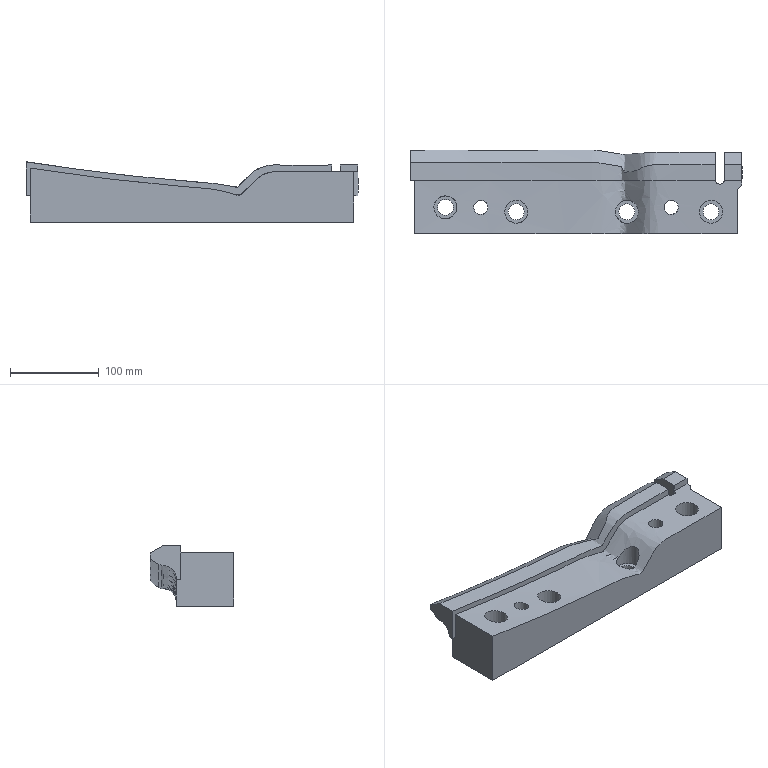Part | NX | features solid 2 | 1 solid | 49 faces | box 377.307 x 94.751 x 68.071 mm | volume 1287517 mm3 | plane 20 | spline 18 | cylinder 11 | commonest cylinder face diameters 18 x4 26 x4 16 x2 10 x1